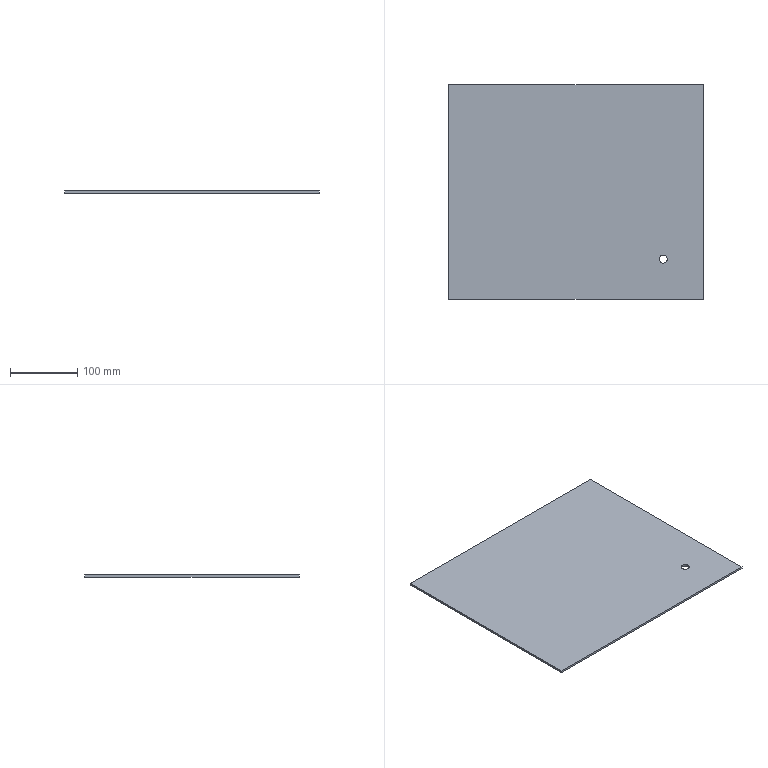Part | SolidWorks | features Extrusion 1, ICE 1 | 1 solid | 8 faces | box 380 x 320 x 3 mm | volume 364461 mm3 | plane 6 | cylinder 2 | commonest cylinder face diameters 12 x2
STEP:
#1=CARTESIAN_POINT('',(124.,-100.,-1.5));
#2=VERTEX_POINT('',#1);
#3=CARTESIAN_POINT('',(136.,-100.,-1.5));
#4=VERTEX_POINT('',#3);
#5=CARTESIAN_POINT('',(130.,-100.,-1.5));
#6=DIRECTION('',(0.,0.,1.));
#7=DIRECTION('',(1.,0.,0.));
#8=AXIS2_PLACEMENT_3D('',#5,#6,#7);
#9=CIRCLE('',#8,6.);
#10=EDGE_CURVE('',#2,#4,#9,.T.);
#11=ORIENTED_EDGE('',*,*,#10,.F.);
#12=CARTESIAN_POINT('',(124.,-100.,1.5));
#13=VERTEX_POINT('',#12);
#14=CARTESIAN_POINT('',(124.,-100.,-11.5));
#15=DIRECTION('',(0.,0.,1.));
#16=VECTOR('',#15,1000.);
#17=LINE('',#14,#16);
#18=EDGE_CURVE('',#2,#13,#17,.T.);
#19=ORIENTED_EDGE('',*,*,#18,.T.);
#20=CARTESIAN_POINT('',(136.,-100.,1.5));
#21=VERTEX_POINT('',#20);
#22=CARTESIAN_POINT('',(130.,-100.,1.5));
#23=DIRECTION('',(0.,0.,1.));
#24=DIRECTION('',(1.,0.,0.));
#25=AXIS2_PLACEMENT_3D('',#22,#23,#24);
#26=CIRCLE('',#25,6.);
#27=EDGE_CURVE('',#13,#21,#26,.T.);
#28=ORIENTED_EDGE('',*,*,#27,.T.);
#29=CARTESIAN_POINT('',(136.,-100.,-11.5));
#30=DIRECTION('',(0.,0.,1.));
#31=VECTOR('',#30,1000.);
#32=LINE('',#29,#31);
#33=EDGE_CURVE('',#4,#21,#32,.T.);
#34=ORIENTED_EDGE('',*,*,#33,.F.);
#35=EDGE_LOOP('',(#11,#19,#28,#34));
#36=FACE_OUTER_BOUND('',#35,.T.);
#37=CARTESIAN_POINT('',(130.,-100.,-11.5));
#38=DIRECTION('',(0.,0.,1.));
#39=DIRECTION('',(1.,0.,0.));
#40=AXIS2_PLACEMENT_3D('',#37,#38,#39);
#41=CYLINDRICAL_SURFACE('',#40,6.);
#42=ADVANCED_FACE('',(#36),#41,.F.);
#43=CARTESIAN_POINT('',(-190.,160.,1.5));
#44=VERTEX_POINT('',#43);
#45=CARTESIAN_POINT('',(-190.,-160.,1.5));
#46=VERTEX_POINT('',#45);
#47=CARTESIAN_POINT('',(-190.,160.,1.5));
#48=DIRECTION('',(0.,-1.,0.));
#49=VECTOR('',#48,1000.);
#50=LINE('',#47,#49);
#51=EDGE_CURVE('',#44,#46,#50,.T.);
#52=ORIENTED_EDGE('',*,*,#51,.F.);
#53=CARTESIAN_POINT('',(-190.,160.,-1.5));
#54=VERTEX_POINT('',#53);
#55=CARTESIAN_POINT('',(-190.,160.,-1.5));
#56=DIRECTION('',(0.,0.,1.));
#57=VECTOR('',#56,1000.);
#58=LINE('',#55,#57);
#59=EDGE_CURVE('',#54,#44,#58,.T.);
#60=ORIENTED_EDGE('',*,*,#59,.F.);
#61=CARTESIAN_POINT('',(-190.,-160.,-1.5));
#62=VERTEX_POINT('',#61);
#63=CARTESIAN_POINT('',(-190.,160.,-1.5));
#64=DIRECTION('',(0.,-1.,0.));
#65=VECTOR('',#64,1000.);
#66=LINE('',#63,#65);
#67=EDGE_CURVE('',#54,#62,#66,.T.);
#68=ORIENTED_EDGE('',*,*,#67,.T.);
#69=CARTESIAN_POINT('',(-190.,-160.,-1.5));
#70=DIRECTION('',(0.,0.,1.));
#71=VECTOR('',#70,1000.);
#72=LINE('',#69,#71);
#73=EDGE_CURVE('',#62,#46,#72,.T.);
#74=ORIENTED_EDGE('',*,*,#73,.T.);
#75=EDGE_LOOP('',(#52,#60,#68,#74));
#76=FACE_OUTER_BOUND('',#75,.T.);
#77=CARTESIAN_POINT('',(-190.,160.,-1.5));
#78=DIRECTION('',(-1.,0.,0.));
#79=DIRECTION('',(0.,0.,1.));
#80=AXIS2_PLACEMENT_3D('',#77,#78,#79);
#81=PLANE('',#80);
#82=ADVANCED_FACE('',(#76),#81,.T.);
#83=CARTESIAN_POINT('',(190.,160.,1.5));
#84=VERTEX_POINT('',#83);
#85=CARTESIAN_POINT('',(190.,160.,1.5));
#86=DIRECTION('',(-1.,0.,0.));
#87=VECTOR('',#86,1000.);
#88=LINE('',#85,#87);
#89=EDGE_CURVE('',#84,#44,#88,.T.);
#90=ORIENTED_EDGE('',*,*,#89,.F.);
#91=CARTESIAN_POINT('',(190.,160.,-1.5));
#92=VERTEX_POINT('',#91);
#93=CARTESIAN_POINT('',(190.,160.,-1.5));
#94=DIRECTION('',(0.,0.,1.));
#95=VECTOR('',#94,1000.);
#96=LINE('',#93,#95);
#97=EDGE_CURVE('',#92,#84,#96,.T.);
#98=ORIENTED_EDGE('',*,*,#97,.F.);
#99=CARTESIAN_POINT('',(190.,160.,-1.5));
#100=DIRECTION('',(-1.,0.,0.));
#101=VECTOR('',#100,1000.);
#102=LINE('',#99,#101);
#103=EDGE_CURVE('',#92,#54,#102,.T.);
#104=ORIENTED_EDGE('',*,*,#103,.T.);
#105=ORIENTED_EDGE('',*,*,#59,.T.);
#106=EDGE_LOOP('',(#90,#98,#104,#105));
#107=FACE_OUTER_BOUND('',#106,.T.);
#108=CARTESIAN_POINT('',(190.,160.,-1.5));
#109=DIRECTION('',(0.,1.,0.));
#110=DIRECTION('',(0.,0.,1.));
#111=AXIS2_PLACEMENT_3D('',#108,#109,#110);
#112=PLANE('',#111);
#113=ADVANCED_FACE('',(#107),#112,.T.);
#114=CARTESIAN_POINT('',(190.,-160.,1.5));
#115=VERTEX_POINT('',#114);
#116=CARTESIAN_POINT('',(190.,-160.,1.5));
#117=DIRECTION('',(0.,1.,0.));
#118=VECTOR('',#117,1000.);
#119=LINE('',#116,#118);
#120=EDGE_CURVE('',#115,#84,#119,.T.);
#121=ORIENTED_EDGE('',*,*,#120,.F.);
#122=CARTESIAN_POINT('',(190.,-160.,-1.5));
#123=VERTEX_POINT('',#122);
#124=CARTESIAN_POINT('',(190.,-160.,-1.5));
#125=DIRECTION('',(0.,0.,1.));
#126=VECTOR('',#125,1000.);
#127=LINE('',#124,#126);
#128=EDGE_CURVE('',#123,#115,#127,.T.);
#129=ORIENTED_EDGE('',*,*,#128,.F.);
#130=CARTESIAN_POINT('',(190.,-160.,-1.5));
#131=DIRECTION('',(0.,1.,0.));
#132=VECTOR('',#131,1000.);
#133=LINE('',#130,#132);
#134=EDGE_CURVE('',#123,#92,#133,.T.);
#135=ORIENTED_EDGE('',*,*,#134,.T.);
#136=ORIENTED_EDGE('',*,*,#97,.T.);
#137=EDGE_LOOP('',(#121,#129,#135,#136));
#138=FACE_OUTER_BOUND('',#137,.T.);
#139=CARTESIAN_POINT('',(190.,-160.,-1.5));
#140=DIRECTION('',(1.,0.,0.));
#141=DIRECTION('',(0.,0.,-1.));
#142=AXIS2_PLACEMENT_3D('',#139,#140,#141);
#143=PLANE('',#142);
#144=ADVANCED_FACE('',(#138),#143,.T.);
#145=CARTESIAN_POINT('',(-190.,-160.,1.5));
#146=DIRECTION('',(1.,0.,0.));
#147=VECTOR('',#146,1000.);
#148=LINE('',#145,#147);
#149=EDGE_CURVE('',#46,#115,#148,.T.);
#150=ORIENTED_EDGE('',*,*,#149,.F.);
#151=ORIENTED_EDGE('',*,*,#73,.F.);
#152=CARTESIAN_POINT('',(-190.,-160.,-1.5));
#153=DIRECTION('',(1.,0.,0.));
#154=VECTOR('',#153,1000.);
#155=LINE('',#152,#154);
#156=EDGE_CURVE('',#62,#123,#155,.T.);
#157=ORIENTED_EDGE('',*,*,#156,.T.);
#158=ORIENTED_EDGE('',*,*,#128,.T.);
#159=EDGE_LOOP('',(#150,#151,#157,#158));
#160=FACE_OUTER_BOUND('',#159,.T.);
#161=CARTESIAN_POINT('',(-190.,-160.,-1.5));
#162=DIRECTION('',(0.,-1.,0.));
#163=DIRECTION('',(0.,0.,-1.));
#164=AXIS2_PLACEMENT_3D('',#161,#162,#163);
#165=PLANE('',#164);
#166=ADVANCED_FACE('',(#160),#165,.T.);
#167=CARTESIAN_POINT('',(130.,-100.,-1.5));
#168=DIRECTION('',(0.,0.,1.));
#169=DIRECTION('',(1.,0.,0.));
#170=AXIS2_PLACEMENT_3D('',#167,#168,#169);
#171=CIRCLE('',#170,6.);
#172=EDGE_CURVE('',#4,#2,#171,.T.);
#173=ORIENTED_EDGE('',*,*,#172,.T.);
#174=ORIENTED_EDGE('',*,*,#10,.T.);
#175=EDGE_LOOP('',(#173,#174));
#176=FACE_BOUND('',#175,.T.);
#177=ORIENTED_EDGE('',*,*,#67,.F.);
#178=ORIENTED_EDGE('',*,*,#103,.F.);
#179=ORIENTED_EDGE('',*,*,#134,.F.);
#180=ORIENTED_EDGE('',*,*,#156,.F.);
#181=EDGE_LOOP('',(#177,#178,#179,#180));
#182=FACE_OUTER_BOUND('',#181,.T.);
#183=CARTESIAN_POINT('',(0.,0.,-1.5));
#184=DIRECTION('',(0.,0.,1.));
#185=DIRECTION('',(1.,0.,0.));
#186=AXIS2_PLACEMENT_3D('',#183,#184,#185);
#187=PLANE('',#186);
#188=ADVANCED_FACE('',(#176,#182),#187,.F.);
#189=CARTESIAN_POINT('',(130.,-100.,1.5));
#190=DIRECTION('',(0.,0.,1.));
#191=DIRECTION('',(1.,0.,0.));
#192=AXIS2_PLACEMENT_3D('',#189,#190,#191);
#193=CIRCLE('',#192,6.);
#194=EDGE_CURVE('',#21,#13,#193,.T.);
#195=ORIENTED_EDGE('',*,*,#194,.F.);
#196=ORIENTED_EDGE('',*,*,#27,.F.);
#197=EDGE_LOOP('',(#195,#196));
#198=FACE_BOUND('',#197,.T.);
#199=ORIENTED_EDGE('',*,*,#51,.T.);
#200=ORIENTED_EDGE('',*,*,#149,.T.);
#201=ORIENTED_EDGE('',*,*,#120,.T.);
#202=ORIENTED_EDGE('',*,*,#89,.T.);
#203=EDGE_LOOP('',(#199,#200,#201,#202));
#204=FACE_OUTER_BOUND('',#203,.T.);
#205=CARTESIAN_POINT('',(0.,0.,1.5));
#206=DIRECTION('',(0.,0.,1.));
#207=DIRECTION('',(1.,0.,0.));
#208=AXIS2_PLACEMENT_3D('',#205,#206,#207);
#209=PLANE('',#208);
#210=ADVANCED_FACE('',(#198,#204),#209,.T.);
#211=ORIENTED_EDGE('',*,*,#18,.F.);
#212=ORIENTED_EDGE('',*,*,#172,.F.);
#213=ORIENTED_EDGE('',*,*,#33,.T.);
#214=ORIENTED_EDGE('',*,*,#194,.T.);
#215=EDGE_LOOP('',(#211,#212,#213,#214));
#216=FACE_OUTER_BOUND('',#215,.T.);
#217=CARTESIAN_POINT('',(130.,-100.,-11.5));
#218=DIRECTION('',(0.,0.,1.));
#219=DIRECTION('',(1.,0.,0.));
#220=AXIS2_PLACEMENT_3D('',#217,#218,#219);
#221=CYLINDRICAL_SURFACE('',#220,6.);
#222=ADVANCED_FACE('',(#216),#221,.F.);
#223=CLOSED_SHELL('',(#42,#82,#113,#144,#166,#188,#210,#222));
#224=MANIFOLD_SOLID_BREP('',#223);
#225=CARTESIAN_POINT('',(0.,0.,0.));
#226=DIRECTION('',(0.,0.,1.));
#227=DIRECTION('',(1.,0.,0.));
#228=AXIS2_PLACEMENT_3D('',#225,#226,#227);
#229=(LENGTH_UNIT()NAMED_UNIT(*)SI_UNIT(.MILLI.,.METRE.));
#230=UNCERTAINTY_MEASURE_WITH_UNIT(LENGTH_MEASURE(0.00001),#229,'','');
#231=(NAMED_UNIT(*)PLANE_ANGLE_UNIT()SI_UNIT($,.RADIAN.));
#232=(NAMED_UNIT(*)SI_UNIT($,.STERADIAN.)SOLID_ANGLE_UNIT());
#233=(GEOMETRIC_REPRESENTATION_CONTEXT(3)GLOBAL_UNCERTAINTY_ASSIGNED_CONTEXT((#230))GLOBAL_UNIT_ASSIGNED_CONTEXT((#229,#231,#232))REPRESENTATION_CONTEXT('',''));
#234=ADVANCED_BREP_SHAPE_REPRESENTATION('',(#224,#228),#233);